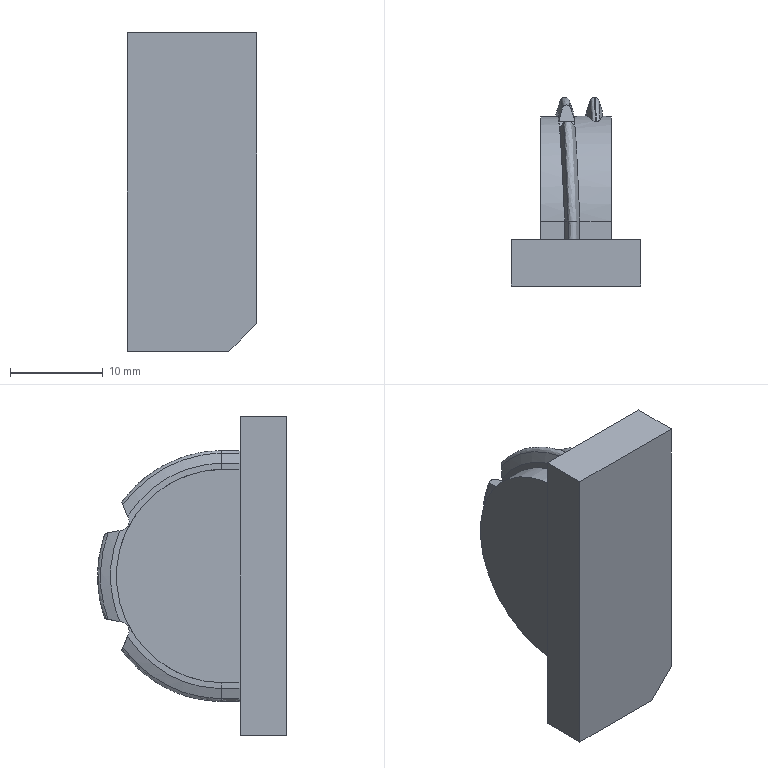NC program | NX | posted with a generic post | part box 13.933 x 20.347 x 34.335 mm
Lines 105534 to 105565 of 105565:
(FIXED_CONTOUR , TOOL : D1.5)
N211006 M6
N211008 G54
N211010 G17 G0 G90 X-7.496 Y0.061 S3000 M3
N211012 G43 Z3. H0
N211014 Z-2.369
N211016 G94 G1 Z-4.369 F500.
N211018 X-6.977 Y0.087 Z-4.013 F2500.
N211020 X-6.458 Y0.113 Z-3.698
N211022 X-5.938 Y0.139 Z-3.418
N211024 X-5.419 Y0.165 Z-3.173
N211026 X-4.9 Y0.191 Z-2.958
N211028 X-4.381 Y0.216 Z-2.771
N211030 X-3.862 Y0.242 Z-2.611
N211032 X-3.343 Y0.268 Z-2.479
N211034 X-2.824 Y0.294 Z-2.371
N211036 X-2.305 Y0.32 Z-2.288
N211038 X-1.786 Y0.346 Z-2.23
N211040 X-1.267 Y0.372 Z-2.194
N211042 X-0.748 Y0.398 Z-2.183
N211044 X0.81 Y0.476
N211046 X0.937 Y0.492 Z-2.184
N211048 X1.478 Y0.604 Z-2.2
N211050 X2.018 Y0.717 Z-2.256
N211052 X2.559 Y0.829 Z-2.328
N211054 X3.099 Y0.942 Z-2.428
N211056 Z-0.428
N211058 G0 Z3.
N211060 M5
N211062 M2